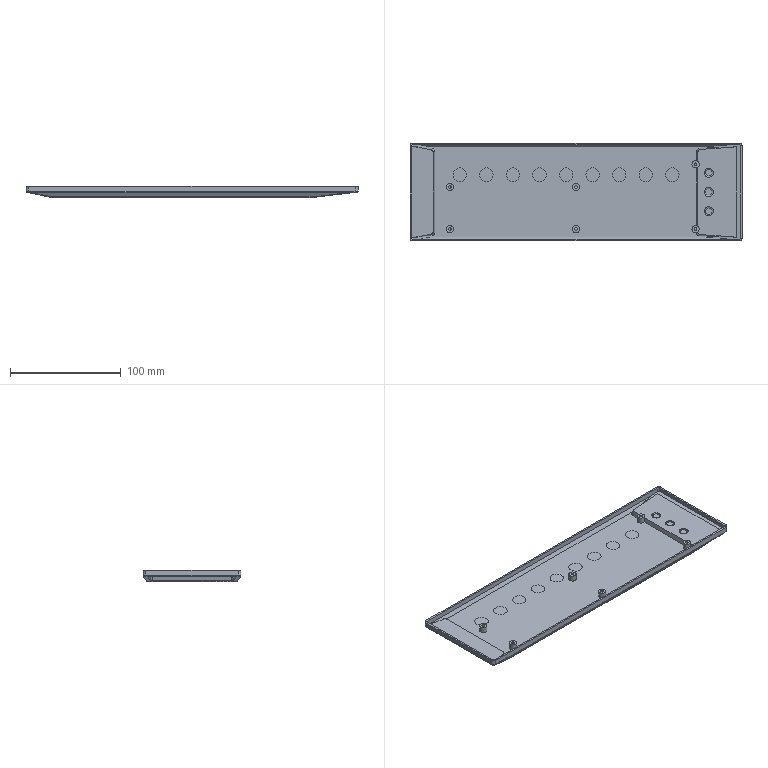NC program | NX | posted with a generic post | part box 300 x 88.5 x 10 mm
Lines 2815 to 3381 of 79950:
(CAVITY_MILL_COPY_COPY_COPY_2 , TOOL : D2)
N5610 T02 M6
N5612 G54
N5614 G17 G0 G90 X-102.412 Y32.208 S9500 M3
N5616 G43 Z30. H2
N5618 Z0.8
N5620 G94 G1 Z-0.2 F1000.
N5622 X-102.466 Y32.222
N5624 G3 X-103.298 Y32.075 R1.
N5626 G1 X-103.845 Y31.691 F1100.
N5628 Y31.022
N5630 G3 X-103.488 Y30.256 R1.
N5632 G1 X-103.445 Y30.22
N5634 Z0.8
N5636 G0 X-101.467 Y31.717 Z0.65
N5638 G1 Z-0.35 F1000.
N5640 X-101.521 Y31.731
N5642 G3 X-102.353 Y31.583 R1.
N5644 G1 X-102.884 Y31.21 F1100.
N5646 X-102.9 Y31.129
N5648 Y30.531
N5650 G3 X-102.543 Y29.765 R1.
N5652 G1 X-102.5 Y29.729
N5654 Z0.65
N5656 G0 X-100.612 Y31.273 Z0.5
N5658 G1 Z-0.5 F1000.
N5660 X-100.666 Y31.287
N5662 G3 X-101.498 Y31.139 R1.
N5664 G1 X-102.045 Y30.755 F1100.
N5666 Y30.087
N5668 G3 X-101.688 Y29.321 R1.
N5670 G1 X-101.645 Y29.285
N5672 Z0.5
N5674 G0 X-100.567 Y31.249 Z0.333
N5676 G1 Z-0.667 F1000.
N5678 X-100.621 Y31.264
N5680 G3 X-101.453 Y31.116 R1.
N5682 G1 X-102. Y30.731 F1100.
N5684 Y30.064
N5686 G3 X-101.643 Y29.297 R1.
N5688 G1 X-101.6 Y29.262
N5690 Z0.333
N5692 G0 X-100.567 Y31.249 Z0.167
N5694 G1 Z-0.833 F1000.
N5696 X-100.621 Y31.264
N5698 G3 X-101.453 Y31.116 R1.
N5700 G1 X-102. Y30.73 F1100.
N5702 Y30.064
N5704 G3 X-101.643 Y29.297 R1.
N5706 G1 X-101.6 Y29.262
N5708 Z0.167
N5710 G0 X-100.567 Y31.249 Z0.
N5712 G1 Z-1. F1000.
N5714 X-100.621 Y31.264
N5716 G3 X-101.453 Y31.116 R1.
N5718 G1 X-102. Y30.729 F1100.
N5720 Y30.064
N5722 G3 X-101.643 Y29.297 R1.
N5724 G1 X-101.6 Y29.262
N5726 Z0.
N5728 G0 Z30.
N5730 X-103.445 Y4.457
N5732 Z0.8
N5734 G1 Z-0.2 F1000.
N5736 X-103.488 Y4.421
N5738 G3 X-103.845 Y3.655 R1.
N5740 G1 Y3.06 F1100.
N5742 X-103.833 Y3.01
N5744 X-103.344 Y2.628
N5746 G3 X-102.52 Y2.437 R1.
N5748 G1 X-102.465 Y2.449
N5750 Z0.8
N5752 G0 X-102.5 Y4.918 Z0.65
N5754 G1 Z-0.35 F1000.
N5756 X-102.543 Y4.882
N5758 G3 X-102.9 Y4.116 R1.
N5760 G1 Y3.48 F1100.
N5762 X-102.399 Y3.089
N5764 G3 X-101.575 Y2.898 R1.
N5766 G1 X-101.52 Y2.91
N5768 Z0.65
N5770 G0 X-101.645 Y5.335 Z0.5
N5772 G1 Z-0.5 F1000.
N5774 X-101.688 Y5.299
N5776 G3 X-102.045 Y4.533 R1.
N5778 G1 Y3.897 F1100.
N5780 X-101.544 Y3.506
N5782 G3 X-100.72 Y3.315 R1.
N5784 G1 X-100.665 Y3.327
N5786 Z0.5
N5788 G0 X-101.6 Y5.357 Z0.333
N5790 G1 Z-0.667 F1000.
N5792 X-101.643 Y5.321
N5794 G3 X-102. Y4.555 R1.
N5796 G1 X-101.999 Y3.919 F1100.
N5798 X-101.499 Y3.527
N5800 G3 X-100.675 Y3.337 R1.
N5802 G1 X-100.62 Y3.349
N5804 Z0.333
N5806 G0 X-101.6 Y5.357 Z0.167
N5808 G1 Z-0.833 F1000.
N5810 X-101.643 Y5.321
N5812 G3 X-102. Y4.555 R1.
N5814 G1 Y3.921 F1100.
N5816 X-101.499 Y3.527
N5818 G3 X-100.675 Y3.337 R1.
N5820 G1 X-100.62 Y3.349
N5822 Z0.167
N5824 G0 X-101.6 Y5.357 Z0.
N5826 G1 Z-1. F1000.
N5828 X-101.643 Y5.321
N5830 G3 X-102. Y4.555 R1.
N5832 G1 Y3.919 F1100.
N5834 X-101.499 Y3.527
N5836 G3 X-100.675 Y3.337 R1.
N5838 G1 X-100.62 Y3.349
N5840 Z0.
N5842 G0 Z30.
N5844 X-111.498 Y-24.101
N5846 Z0.8
N5848 G1 Z-0.2 F1000.
N5850 G3 X-111.014 Y-23.6 R1.
N5852 G2 X-110.098 Y-23. R1. F1100.
N5854 G1 X-15.
N5856 Y-22.5
N5858 X-110.098
N5860 G2 X-111.024 Y-21.878 R1.
N5862 G3 X-111.498 Y-21.364 R1.
N5864 G1 Z0.8
N5866 G0 Z30.
N5868 Y-29.194
N5870 Z0.8
N5872 G1 Z-0.2 F1000.
N5874 G3 X-111.038 Y-28.658 R1.
N5876 G2 X-110.098 Y-28. R1. F1100.
N5878 G1 X-15.
N5880 Y-27.5
N5882 X-110.098
N5884 G2 X-111.023 Y-26.881 R1.
N5886 G3 X-111.498 Y-26.368 R1.
N5888 G1 Z0.8
N5890 G0 Z30.
N5892 Y-34.12
N5894 Z0.8
N5896 G1 Z-0.2 F1000.
N5898 G3 X-111.019 Y-33.612 R1.
N5900 G2 X-110.098 Y-33. R1. F1100.
N5902 G1 X-15.
N5904 Y-32.5
N5906 X-110.098
N5908 G2 X-111.018 Y-31.891 R1.
N5910 G3 X-111.498 Y-31.385 R1.
N5912 G1 Z0.8
N5914 G0 Z30.
N5916 X-7.6 Y-32.05
N5918 Z0.8
N5920 G1 Z-0.2 F1000.
N5922 X-7.643 Y-32.086
N5924 G3 X-8. Y-32.852 R1.
N5926 G1 Y-34. F1100.
N5928 X-6.852
N5930 G3 X-6.086 Y-33.643 R1.
N5932 G1 X-6.05 Y-33.6
N5934 Z0.8
N5936 G0 X-7.6 Y-32.05 Z0.65
N5938 G1 Z-0.35 F1000.
N5940 X-7.643 Y-32.086
N5942 G3 X-8. Y-32.852 R1.
N5944 G1 Y-34. F1100.
N5946 X-6.852
N5948 G3 X-6.086 Y-33.643 R1.
N5950 G1 X-6.05 Y-33.6
N5952 Z0.65
N5954 G0 X-7.6 Y-32.05 Z0.5
N5956 G1 Z-0.5 F1000.
N5958 X-7.643 Y-32.086
N5960 G3 X-8. Y-32.852 R1.
N5962 G1 X-7.999 Y-34. F1100.
N5964 X-6.852
N5966 G3 X-6.086 Y-33.643 R1.
N5968 G1 X-6.05 Y-33.6
N5970 Z0.5
N5972 G0 Z30.
N5974 Y-22.4
N5976 Z0.8
N5978 G1 Z-0.2 F1000.
N5980 X-6.086 Y-22.357
N5982 G3 X-6.852 Y-22. R1.
N5984 G1 X-8. F1100.
N5986 Y-23.148
N5988 G3 X-7.643 Y-23.914 R1.
N5990 G1 X-7.6 Y-23.95
N5992 Z0.8
N5994 G0 X-6.05 Y-22.4 Z0.65
N5996 G1 Z-0.35 F1000.
N5998 X-6.086 Y-22.357
N6000 G3 X-6.852 Y-22. R1.
N6002 G1 X-8. F1100.
N6004 Y-23.148
N6006 G3 X-7.643 Y-23.914 R1.
N6008 G1 X-7.6 Y-23.95
N6010 Z0.65
N6012 G0 X-6.05 Y-22.4 Z0.5
N6014 G1 Z-0.5 F1000.
N6016 X-6.086 Y-22.357
N6018 G3 X-6.852 Y-22. R1.
N6020 G1 X-8. F1100.
N6022 Y-23.148
N6024 G3 X-7.643 Y-23.914 R1.
N6026 G1 X-7.6 Y-23.95
N6028 Z0.5
N6030 G0 Z30.
N6032 X-111.537 Y-11.923
N6034 Z0.8
N6036 G1 Z-0.2 F1000.
N6038 X-111.525 Y-11.933
N6040 G2 X-111.128 Y-12.679 R1.
N6042 G1 X-111.124 Y-12.755 F1100.
N6044 G2 X-111.171 Y-13.01 R0.56
N6046 G3 X-111.018 Y-13.608 R0.5
N6048 G2 X-110.098 Y-13. R1.
N6050 G1 X127.405
N6052 G2 X128.316 Y-13.589 R1.
N6054 G3 X128.457 Y-12.988 R0.5
N6056 G2 X128.458 Y-12.513 R0.56
N6058 G3 X128.318 Y-11.908 R0.5
N6060 G2 X127.405 Y-12.5 R1.
N6062 G1 X-110.098
N6064 G2 X-111.018 Y-11.89 R1.
N6066 G3 X-111.173 Y-12.486 R0.5
N6068 G1 X-111.113 Y-12.573
N6070 X-111.128 Y-12.679
N6072 G2 X-111.444 Y-13.463 R1.
N6074 G1 X-111.544 Y-13.556
N6076 Z0.8
N6078 G0 Z30.
N6080 X128.816 Y-7.748
N6082 Z0.8
N6084 G1 Z-0.2 F1000.
N6086 X128.376 Y-7.781
N6088 G3 X128.332 Y-8.625 R1.
N6090 X128.479 Y-7.993 R0.5 F1100.
N6092 G2 X128.467 Y-7.503 R0.56
N6094 G3 X128.321 Y-6.901 R0.5
N6096 G2 X127.405 Y-7.5 R1.
N6098 G1 X-110.098
N6100 G2 X-111.009 Y-6.911 R1.
N6102 G3 X-111.148 Y-7.514 R0.5
N6104 G2 X-111.146 Y-7.987 R0.56
N6106 G3 X-111.007 Y-8.584 R0.5
N6108 G2 X-110.098 Y-8. R1.
N6110 G1 X127.405
N6112 G2 X128.332 Y-8.625 R1.
N6114 G3 X128.805 Y-9.141 R1.
N6116 G1 Z0.8
N6118 G0 Z30.
N6120 X-111.582 Y-16.959
N6122 Z0.8
N6124 G1 Z-0.2 F1000.
N6126 G2 X-111.207 Y-17.441 R1.
N6128 G1 X-111.189 Y-17.498 F1100.
N6130 X-111.149 Y-17.658
N6132 G2 X-111.179 Y-18.018 R0.56
N6134 G3 X-111.021 Y-18.616 R0.5
N6136 G2 X-110.098 Y-18. R1.
N6138 G1 X127.405
N6140 G2 X128.318 Y-18.592 R1.
N6142 G3 X128.459 Y-17.988 R0.5
N6144 G2 X128.459 Y-17.512 R0.56
N6146 G3 X128.318 Y-16.907 R0.5
N6148 G2 X127.405 Y-17.5 R1.
N6150 G1 X-110.098
N6152 G2 X-111.03 Y-16.863 R1.
N6154 G3 X-111.207 Y-17.441 R0.5
N6156 G2 X-111.278 Y-18.283 R1.
N6158 G1 X-111.499 Y-18.668
N6160 Z0.8
N6162 G0 Z30.
N6164 X-111.547 Y-36.934
N6166 Z0.8
N6168 G1 Z-0.2 F1000.
N6170 G2 X-111.138 Y-37.634 R1.
N6172 G1 X-111.128 Y-37.724 F1100.
N6174 G2 X-111.172 Y-38.011 R0.56
N6176 G3 X-111.018 Y-38.609 R0.5
N6178 G2 X-110.098 Y-38. R1.
N6180 G1 X127.405
N6182 G2 X128.317 Y-38.591 R1.
N6184 G3 X128.458 Y-37.988 R0.5
N6186 G2 X128.459 Y-37.512 R0.56
N6188 G3 X128.318 Y-36.908 R0.5
N6190 G2 X127.405 Y-37.5 R1.
N6192 G1 X-110.098
N6194 G2 X-111.02 Y-36.887 R1.
N6196 G3 X-111.178 Y-37.479 R0.5
N6198 G1 X-111.138 Y-37.634
N6200 G2 X-111.408 Y-38.435 R1.
N6202 G1 X-111.539 Y-38.573
N6204 Z0.8
N6206 G0 Z30.
N6208 X96.05 Y-33.6
N6210 Z0.8
N6212 G1 Z-0.2 F1000.
N6214 X96.086 Y-33.643
N6216 G3 X96.852 Y-34. R1.
N6218 G1 X98. F1100.
N6220 Y-32.852
N6222 G3 X97.643 Y-32.086 R1.
N6224 G1 X97.6 Y-32.05
N6226 Z0.8
N6228 G0 X96.05 Y-33.6 Z0.65
N6230 G1 Z-0.35 F1000.
N6232 X96.086 Y-33.643
N6234 G3 X96.852 Y-34. R1.
N6236 G1 X98. F1100.
N6238 Y-32.852
N6240 G3 X97.643 Y-32.086 R1.
N6242 G1 X97.6 Y-32.05
N6244 Z0.65
N6246 G0 X96.05 Y-33.6 Z0.5
N6248 G1 Z-0.5 F1000.
N6250 X96.086 Y-33.643
N6252 G3 X96.852 Y-34. R1.
N6254 G1 X98. F1100.
N6256 Y-32.852
N6258 G3 X97.643 Y-32.086 R1.
N6260 G1 X97.6 Y-32.05
N6262 Z0.5
N6264 G0 Z30.
N6266 Y-23.951
N6268 Z0.8
N6270 G1 Z-0.2 F1000.
N6272 X97.643 Y-23.915
N6274 G3 X98. Y-23.149 R1.
N6276 G1 Y-22. F1100.
N6278 X96.851
N6280 G3 X96.085 Y-22.357 R1.
N6282 G1 X96.049 Y-22.4
N6284 Z0.8
N6286 G0 X97.6 Y-23.951 Z0.65
N6288 G1 Z-0.35 F1000.
N6290 X97.643 Y-23.915
N6292 G3 X98. Y-23.149 R1.
N6294 G1 Y-22. F1100.
N6296 X96.851
N6298 G3 X96.085 Y-22.357 R1.
N6300 G1 X96.049 Y-22.4
N6302 Z0.65
N6304 G0 X97.6 Y-23.951 Z0.5
N6306 G1 Z-0.5 F1000.
N6308 X97.643 Y-23.916
N6310 G3 X98. Y-23.149 R1.
N6312 G1 Y-22. F1100.
N6314 X96.851
N6316 G3 X96.084 Y-22.357 R1.
N6318 G1 X96.049 Y-22.4
N6320 Z0.5
N6322 G0 Z30.
N6324 X128.805 Y-26.405
N6326 Z0.8
N6328 G1 Z-0.2 F1000.
N6330 G3 X128.32 Y-26.904 R1.
N6332 G2 X127.405 Y-27.5 R1. F1100.
N6334 G1 X105. Y-27.501
N6336 Y-28.
N6338 X127.405
N6340 G2 X128.324 Y-28.606 R1.
N6342 G3 X128.805 Y-29.111 R1.
N6344 G1 Z0.8
N6346 G0 Z30.
N6348 Y-31.249
N6350 Z0.8
N6352 G1 Z-0.2 F1000.
N6354 G3 X128.357 Y-31.806 R1.
N6356 G2 X127.405 Y-32.5 R1. F1100.
N6358 G1 X105.
N6360 Y-33.
N6362 X127.405
N6364 G2 X128.36 Y-33.704 R1.
N6366 G3 X128.805 Y-34.267 R1.
N6368 G1 Z0.8
N6370 G0 Z30.
N6372 Y-21.414
N6374 Z0.8
N6376 G1 Z-0.2 F1000.
N6378 G3 X128.317 Y-21.91 R1.
N6380 G2 X127.405 Y-22.5 R1. F1100.
N6382 G1 X105.
N6384 Y-23.
N6386 X127.405
N6388 G2 X128.318 Y-23.592 R1.
N6390 G3 X128.805 Y-24.089 R1.
N6392 G1 Z0.8
N6394 G0 Z30.
N6396 X115.642 Y-0.795
N6398 Z0.8
N6400 G1 Z-0.2 F1000.
N6402 X115.678 Y-0.838
N6404 G3 X116.444 Y-1.195 R1.
N6406 G1 X116.955 F1100.
N6408 X117.095 Y-1.083
N6410 X117.346 Y-0.864
N6412 G3 X117.69 Y-0.092 R1.
N6414 G1 X117.689 Y-0.036
N6416 Z0.8
N6418 G0 X115.288 Y0.15 Z0.65
N6420 G1 Z-0.35 F1000.
N6422 X115.324 Y0.107
N6424 G3 X116.09 Y-0.25 R1.
N6426 G1 X116.613 F1100.
N6428 X117.007 Y0.093
N6430 G3 X117.351 Y0.865 R1.
N6432 G1 X117.35 Y0.921
N6434 Z0.65
N6436 G0 X114.969 Y1.005 Z0.5
N6438 G1 Z-0.5 F1000.
N6440 X115.005 Y0.962
N6442 G3 X115.771 Y0.605 R1.
N6444 G1 X116.293 F1100.
N6446 X116.687 Y0.948
N6448 G3 X117.031 Y1.72 R1.
N6450 G1 X117.03 Y1.776
N6452 Z0.5
N6454 G0 X114.952 Y1.05 Z0.333
N6456 G1 Z-0.667 F1000.
N6458 X114.988 Y1.007
N6460 G3 X115.754 Y0.65 R1.
N6462 G1 X116.276 F1100.
N6464 X116.67 Y0.993
N6466 G3 X117.014 Y1.765 R1.
N6468 G1 X117.013 Y1.821
N6470 Z0.333
N6472 G0 X114.952 Y1.05 Z0.167
N6474 G1 Z-0.833 F1000.
N6476 X114.988 Y1.007
N6478 G3 X115.754 Y0.65 R1.
N6480 G1 X116.276 F1100.
N6482 X116.67 Y0.993
N6484 G3 X117.014 Y1.765 R1.
N6486 G1 X117.013 Y1.821
N6488 Z0.167
N6490 G0 X114.952 Y1.05 Z0.
N6492 G1 Z-1. F1000.
N6494 X114.988 Y1.007
N6496 G3 X115.754 Y0.65 R1.
N6498 G1 X116.276 F1100.
N6500 X116.67 Y0.993
N6502 G3 X117.014 Y1.765 R1.
N6504 G1 X117.013 Y1.821
N6506 Z0.
N6508 G0 Z30.
N6510 X120.522 Y2.427
N6512 Z0.8
N6514 G1 Z-0.2 F1000.
N6516 X120.577 Y2.418
N6518 G3 X121.39 Y2.651 R1.
N6520 G1 X121.845 Y3.047 F1100.
N6522 Y3.65
N6524 G3 X121.488 Y4.417 R1.
N6526 G1 X121.445 Y4.452
N6528 Z0.8
N6530 G0 X119.576 Y2.856 Z0.65
N6532 G1 Z-0.35 F1000.
N6534 X119.632 Y2.848
N6536 G3 X120.444 Y3.081 R1.
N6538 G1 X120.9 Y3.477 F1100.
N6540 Y4.081
N6542 G3 X120.543 Y4.847 R1.
N6544 G1 X120.5 Y4.883
N6546 Z0.65
N6548 G0 X118.721 Y3.246 Z0.5
N6550 G1 Z-0.5 F1000.
N6552 X118.777 Y3.237
N6554 G3 X119.589 Y3.47 R1.
N6556 G1 X120.045 Y3.867 F1100.
N6558 Y4.471
N6560 G3 X119.688 Y5.237 R1.
N6562 G1 X119.645 Y5.273
N6564 Z0.5
N6566 G0 X118.676 Y3.267 Z0.333
N6568 G1 Z-0.667 F1000.
N6570 X118.732 Y3.258
N6572 G3 X119.544 Y3.491 R1.
N6574 G1 X120. Y3.887 F1100.
N6576 Y4.491
N6578 G3 X119.643 Y5.257 R1.
N6580 G1 X119.6 Y5.293
N6582 Z0.333
N6584 G0 X118.676 Y3.267 Z0.167
N6586 G1 Z-0.833 F1000.
N6588 X118.732 Y3.258
N6590 G3 X119.544 Y3.491 R1.
N6592 G1 X120. Y3.887 F1100.
N6594 Y4.491
N6596 G3 X119.643 Y5.257 R1.
N6598 G1 X119.6 Y5.293
N6600 Z0.167
N6602 G0 X118.676 Y3.267 Z0.
N6604 G1 Z-1. F1000.
N6606 X118.732 Y3.258
N6608 G3 X119.544 Y3.491 R1.
N6610 G1 X120. Y3.887 F1100.
N6612 Y4.491
N6614 G3 X119.643 Y5.257 R1.
N6616 G1 X119.6 Y5.293
N6618 Z0.
N6620 G0 Z30.
N6622 X121.445 Y30.225
N6624 Z0.8
N6626 G1 Z-0.2 F1000.
N6628 X121.488 Y30.261
N6630 G3 X121.845 Y31.027 R1.
N6632 G1 Y31.664 F1100.
N6634 X121.344 Y32.055
N6636 G3 X120.52 Y32.245 R1.
N6638 G1 X120.465 Y32.234
N6640 Z0.8
N6642 G0 X120.5 Y29.765 Z0.65
N6644 G1 Z-0.35 F1000.
N6646 X120.543 Y29.8
N6648 G3 X120.9 Y30.566 R1.
N6650 G1 Y31.149 F1100.
N6652 X120.868 Y31.228
N6654 X120.399 Y31.594
N6656 G3 X119.575 Y31.784 R1.
N6658 G1 X119.52 Y31.773
N6660 Z0.65
N6662 G0 X119.645 Y29.348 Z0.5
N6664 G1 Z-0.5 F1000.
N6666 X119.688 Y29.383
N6668 G3 X120.045 Y30.149 R1.
N6670 G1 Y30.786 F1100.
N6672 X119.544 Y31.177
N6674 G3 X118.72 Y31.367 R1.
N6676 G1 X118.665 Y31.356
N6678 Z0.5
N6680 G0 X119.6 Y29.326 Z0.333
N6682 G1 Z-0.667 F1000.
N6684 X119.643 Y29.361
N6686 G3 X120. Y30.128 R1.
N6688 G1 Y30.764 F1100.
N6690 X119.499 Y31.155
N6692 G3 X118.675 Y31.345 R1.
N6694 G1 X118.62 Y31.334
N6696 Z0.333
N6698 G0 X119.6 Y29.326 Z0.167
N6700 G1 Z-0.833 F1000.
N6702 X119.643 Y29.361
N6704 G3 X120. Y30.128 R1.
N6706 G1 Y30.764 F1100.
N6708 X119.499 Y31.155
N6710 G3 X118.675 Y31.345 R1.
N6712 G1 X118.62 Y31.334
N6714 Z0.167
N6716 G0 X119.6 Y29.326 Z0.
N6718 G1 Z-1. F1000.
N6720 X119.643 Y29.361
N6722 G3 X120. Y30.128 R1.
N6724 G1 Y30.764 F1100.
N6726 X119.499 Y31.155
N6728 G3 X118.675 Y31.345 R1.
N6730 G1 X118.62 Y31.334
N6732 Z0.
N6734 G0 Z30.
N6736 M5